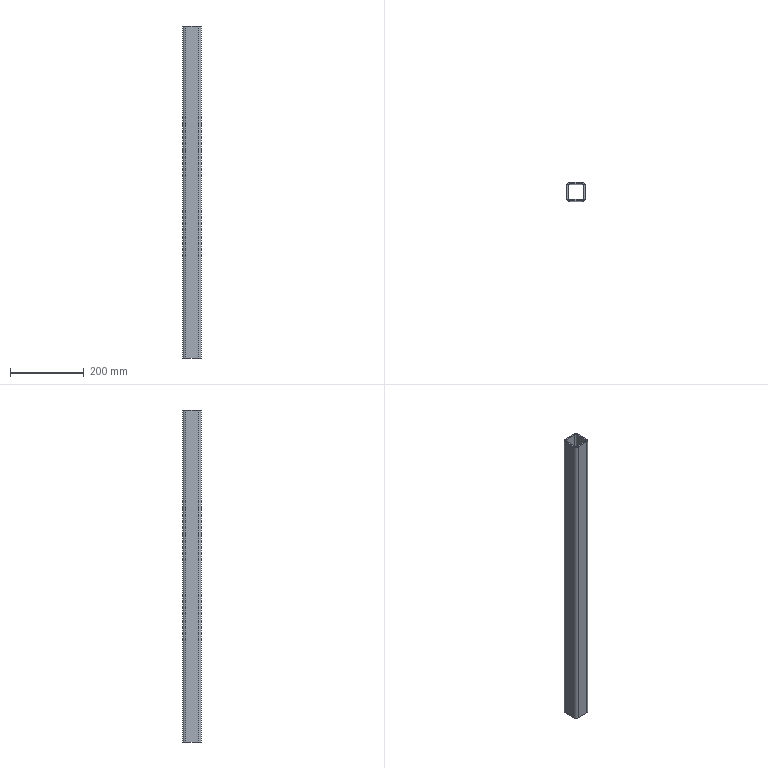Part | SolidWorks | features Extrusion 1 | 1 solid | 18 faces | box 50 x 50 x 900 mm | volume 625317 mm3 | plane 10 | cylinder 8 | commonest cylinder face diameters 8 x4 16 x4
STEP:
#1=CARTESIAN_POINT('',(17.,-25.,450.));
#2=VERTEX_POINT('',#1);
#3=CARTESIAN_POINT('',(25.,-17.,450.));
#4=VERTEX_POINT('',#3);
#5=CARTESIAN_POINT('',(17.,-17.,450.));
#6=DIRECTION('',(0.,0.,1.));
#7=DIRECTION('',(1.,0.,0.));
#8=AXIS2_PLACEMENT_3D('',#5,#6,#7);
#9=CIRCLE('',#8,8.);
#10=EDGE_CURVE('',#2,#4,#9,.T.);
#11=ORIENTED_EDGE('',*,*,#10,.T.);
#12=CARTESIAN_POINT('',(25.,17.,450.));
#13=VERTEX_POINT('',#12);
#14=CARTESIAN_POINT('',(25.,-17.,450.));
#15=DIRECTION('',(0.,1.,0.));
#16=VECTOR('',#15,1000.);
#17=LINE('',#14,#16);
#18=EDGE_CURVE('',#4,#13,#17,.T.);
#19=ORIENTED_EDGE('',*,*,#18,.T.);
#20=CARTESIAN_POINT('',(17.,25.,450.));
#21=VERTEX_POINT('',#20);
#22=CARTESIAN_POINT('',(17.,17.,450.));
#23=DIRECTION('',(0.,0.,1.));
#24=DIRECTION('',(-1.,0.,0.));
#25=AXIS2_PLACEMENT_3D('',#22,#23,#24);
#26=CIRCLE('',#25,8.);
#27=EDGE_CURVE('',#13,#21,#26,.T.);
#28=ORIENTED_EDGE('',*,*,#27,.T.);
#29=CARTESIAN_POINT('',(-17.,25.,450.));
#30=VERTEX_POINT('',#29);
#31=CARTESIAN_POINT('',(-17.,25.,450.));
#32=DIRECTION('',(-1.,0.,0.));
#33=VECTOR('',#32,1000.);
#34=LINE('',#31,#33);
#35=EDGE_CURVE('',#21,#30,#34,.T.);
#36=ORIENTED_EDGE('',*,*,#35,.T.);
#37=CARTESIAN_POINT('',(-25.,17.,450.));
#38=VERTEX_POINT('',#37);
#39=CARTESIAN_POINT('',(-17.,17.,450.));
#40=DIRECTION('',(0.,0.,1.));
#41=DIRECTION('',(-1.,0.,0.));
#42=AXIS2_PLACEMENT_3D('',#39,#40,#41);
#43=CIRCLE('',#42,8.);
#44=EDGE_CURVE('',#30,#38,#43,.T.);
#45=ORIENTED_EDGE('',*,*,#44,.T.);
#46=CARTESIAN_POINT('',(-25.,-17.,450.));
#47=VERTEX_POINT('',#46);
#48=CARTESIAN_POINT('',(-25.,-17.,450.));
#49=DIRECTION('',(0.,-1.,0.));
#50=VECTOR('',#49,1000.);
#51=LINE('',#48,#50);
#52=EDGE_CURVE('',#38,#47,#51,.T.);
#53=ORIENTED_EDGE('',*,*,#52,.T.);
#54=CARTESIAN_POINT('',(-17.,-25.,450.));
#55=VERTEX_POINT('',#54);
#56=CARTESIAN_POINT('',(-17.,-17.,450.));
#57=DIRECTION('',(0.,0.,1.));
#58=DIRECTION('',(-1.,0.,0.));
#59=AXIS2_PLACEMENT_3D('',#56,#57,#58);
#60=CIRCLE('',#59,8.);
#61=EDGE_CURVE('',#47,#55,#60,.T.);
#62=ORIENTED_EDGE('',*,*,#61,.T.);
#63=CARTESIAN_POINT('',(-17.,-25.,450.));
#64=DIRECTION('',(1.,0.,0.));
#65=VECTOR('',#64,1000.);
#66=LINE('',#63,#65);
#67=EDGE_CURVE('',#55,#2,#66,.T.);
#68=ORIENTED_EDGE('',*,*,#67,.T.);
#69=EDGE_LOOP('',(#11,#19,#28,#36,#45,#53,#62,#68));
#70=FACE_OUTER_BOUND('',#69,.T.);
#71=CARTESIAN_POINT('',(-21.,17.,450.));
#72=VERTEX_POINT('',#71);
#73=CARTESIAN_POINT('',(-21.,-17.,450.));
#74=VERTEX_POINT('',#73);
#75=CARTESIAN_POINT('',(-21.,-17.,450.));
#76=DIRECTION('',(0.,-1.,0.));
#77=VECTOR('',#76,1000.);
#78=LINE('',#75,#77);
#79=EDGE_CURVE('',#72,#74,#78,.T.);
#80=ORIENTED_EDGE('',*,*,#79,.F.);
#81=CARTESIAN_POINT('',(-17.,21.,450.));
#82=VERTEX_POINT('',#81);
#83=CARTESIAN_POINT('',(-17.,17.,450.));
#84=DIRECTION('',(0.,0.,1.));
#85=DIRECTION('',(-1.,0.,0.));
#86=AXIS2_PLACEMENT_3D('',#83,#84,#85);
#87=CIRCLE('',#86,4.);
#88=EDGE_CURVE('',#82,#72,#87,.T.);
#89=ORIENTED_EDGE('',*,*,#88,.F.);
#90=CARTESIAN_POINT('',(17.,21.,450.));
#91=VERTEX_POINT('',#90);
#92=CARTESIAN_POINT('',(-17.,21.,450.));
#93=DIRECTION('',(-1.,0.,0.));
#94=VECTOR('',#93,1000.);
#95=LINE('',#92,#94);
#96=EDGE_CURVE('',#91,#82,#95,.T.);
#97=ORIENTED_EDGE('',*,*,#96,.F.);
#98=CARTESIAN_POINT('',(21.,17.,450.));
#99=VERTEX_POINT('',#98);
#100=CARTESIAN_POINT('',(17.,17.,450.));
#101=DIRECTION('',(0.,0.,1.));
#102=DIRECTION('',(-1.,0.,0.));
#103=AXIS2_PLACEMENT_3D('',#100,#101,#102);
#104=CIRCLE('',#103,4.);
#105=EDGE_CURVE('',#99,#91,#104,.T.);
#106=ORIENTED_EDGE('',*,*,#105,.F.);
#107=CARTESIAN_POINT('',(21.,-17.,450.));
#108=VERTEX_POINT('',#107);
#109=CARTESIAN_POINT('',(21.,-17.,450.));
#110=DIRECTION('',(0.,1.,0.));
#111=VECTOR('',#110,1000.);
#112=LINE('',#109,#111);
#113=EDGE_CURVE('',#108,#99,#112,.T.);
#114=ORIENTED_EDGE('',*,*,#113,.F.);
#115=CARTESIAN_POINT('',(17.,-21.,450.));
#116=VERTEX_POINT('',#115);
#117=CARTESIAN_POINT('',(17.,-17.,450.));
#118=DIRECTION('',(0.,0.,1.));
#119=DIRECTION('',(1.,0.,0.));
#120=AXIS2_PLACEMENT_3D('',#117,#118,#119);
#121=CIRCLE('',#120,4.);
#122=EDGE_CURVE('',#116,#108,#121,.T.);
#123=ORIENTED_EDGE('',*,*,#122,.F.);
#124=CARTESIAN_POINT('',(-17.,-21.,450.));
#125=VERTEX_POINT('',#124);
#126=CARTESIAN_POINT('',(-17.,-21.,450.));
#127=DIRECTION('',(1.,0.,0.));
#128=VECTOR('',#127,1000.);
#129=LINE('',#126,#128);
#130=EDGE_CURVE('',#125,#116,#129,.T.);
#131=ORIENTED_EDGE('',*,*,#130,.F.);
#132=CARTESIAN_POINT('',(-17.,-17.,450.));
#133=DIRECTION('',(0.,0.,1.));
#134=DIRECTION('',(-1.,0.,0.));
#135=AXIS2_PLACEMENT_3D('',#132,#133,#134);
#136=CIRCLE('',#135,4.);
#137=EDGE_CURVE('',#74,#125,#136,.T.);
#138=ORIENTED_EDGE('',*,*,#137,.F.);
#139=EDGE_LOOP('',(#80,#89,#97,#106,#114,#123,#131,#138));
#140=FACE_BOUND('',#139,.T.);
#141=CARTESIAN_POINT('',(17.,-17.,450.));
#142=DIRECTION('',(0.,0.,1.));
#143=DIRECTION('',(1.,0.,0.));
#144=AXIS2_PLACEMENT_3D('',#141,#142,#143);
#145=PLANE('',#144);
#146=ADVANCED_FACE('',(#70,#140),#145,.T.);
#147=CARTESIAN_POINT('',(17.,-25.,-450.));
#148=VERTEX_POINT('',#147);
#149=CARTESIAN_POINT('',(25.,-17.,-450.));
#150=VERTEX_POINT('',#149);
#151=CARTESIAN_POINT('',(17.,-17.,-450.));
#152=DIRECTION('',(0.,0.,1.));
#153=DIRECTION('',(1.,0.,0.));
#154=AXIS2_PLACEMENT_3D('',#151,#152,#153);
#155=CIRCLE('',#154,8.);
#156=EDGE_CURVE('',#148,#150,#155,.T.);
#157=ORIENTED_EDGE('',*,*,#156,.F.);
#158=CARTESIAN_POINT('',(-17.,-25.,-450.));
#159=VERTEX_POINT('',#158);
#160=CARTESIAN_POINT('',(-17.,-25.,-450.));
#161=DIRECTION('',(1.,0.,0.));
#162=VECTOR('',#161,1000.);
#163=LINE('',#160,#162);
#164=EDGE_CURVE('',#159,#148,#163,.T.);
#165=ORIENTED_EDGE('',*,*,#164,.F.);
#166=CARTESIAN_POINT('',(-25.,-17.,-450.));
#167=VERTEX_POINT('',#166);
#168=CARTESIAN_POINT('',(-17.,-17.,-450.));
#169=DIRECTION('',(0.,0.,1.));
#170=DIRECTION('',(-1.,0.,0.));
#171=AXIS2_PLACEMENT_3D('',#168,#169,#170);
#172=CIRCLE('',#171,8.);
#173=EDGE_CURVE('',#167,#159,#172,.T.);
#174=ORIENTED_EDGE('',*,*,#173,.F.);
#175=CARTESIAN_POINT('',(-25.,17.,-450.));
#176=VERTEX_POINT('',#175);
#177=CARTESIAN_POINT('',(-25.,-17.,-450.));
#178=DIRECTION('',(0.,-1.,0.));
#179=VECTOR('',#178,1000.);
#180=LINE('',#177,#179);
#181=EDGE_CURVE('',#176,#167,#180,.T.);
#182=ORIENTED_EDGE('',*,*,#181,.F.);
#183=CARTESIAN_POINT('',(-17.,25.,-450.));
#184=VERTEX_POINT('',#183);
#185=CARTESIAN_POINT('',(-17.,17.,-450.));
#186=DIRECTION('',(0.,0.,1.));
#187=DIRECTION('',(-1.,0.,0.));
#188=AXIS2_PLACEMENT_3D('',#185,#186,#187);
#189=CIRCLE('',#188,8.);
#190=EDGE_CURVE('',#184,#176,#189,.T.);
#191=ORIENTED_EDGE('',*,*,#190,.F.);
#192=CARTESIAN_POINT('',(17.,25.,-450.));
#193=VERTEX_POINT('',#192);
#194=CARTESIAN_POINT('',(-17.,25.,-450.));
#195=DIRECTION('',(-1.,0.,0.));
#196=VECTOR('',#195,1000.);
#197=LINE('',#194,#196);
#198=EDGE_CURVE('',#193,#184,#197,.T.);
#199=ORIENTED_EDGE('',*,*,#198,.F.);
#200=CARTESIAN_POINT('',(25.,17.,-450.));
#201=VERTEX_POINT('',#200);
#202=CARTESIAN_POINT('',(17.,17.,-450.));
#203=DIRECTION('',(0.,0.,1.));
#204=DIRECTION('',(-1.,0.,0.));
#205=AXIS2_PLACEMENT_3D('',#202,#203,#204);
#206=CIRCLE('',#205,8.);
#207=EDGE_CURVE('',#201,#193,#206,.T.);
#208=ORIENTED_EDGE('',*,*,#207,.F.);
#209=CARTESIAN_POINT('',(25.,-17.,-450.));
#210=DIRECTION('',(0.,1.,0.));
#211=VECTOR('',#210,1000.);
#212=LINE('',#209,#211);
#213=EDGE_CURVE('',#150,#201,#212,.T.);
#214=ORIENTED_EDGE('',*,*,#213,.F.);
#215=EDGE_LOOP('',(#157,#165,#174,#182,#191,#199,#208,#214));
#216=FACE_OUTER_BOUND('',#215,.T.);
#217=CARTESIAN_POINT('',(-17.,21.,-450.));
#218=VERTEX_POINT('',#217);
#219=CARTESIAN_POINT('',(-21.,17.,-450.));
#220=VERTEX_POINT('',#219);
#221=CARTESIAN_POINT('',(-17.,17.,-450.));
#222=DIRECTION('',(0.,0.,1.));
#223=DIRECTION('',(-1.,0.,0.));
#224=AXIS2_PLACEMENT_3D('',#221,#222,#223);
#225=CIRCLE('',#224,4.);
#226=EDGE_CURVE('',#218,#220,#225,.T.);
#227=ORIENTED_EDGE('',*,*,#226,.T.);
#228=CARTESIAN_POINT('',(-21.,-17.,-450.));
#229=VERTEX_POINT('',#228);
#230=CARTESIAN_POINT('',(-21.,-17.,-450.));
#231=DIRECTION('',(0.,-1.,0.));
#232=VECTOR('',#231,1000.);
#233=LINE('',#230,#232);
#234=EDGE_CURVE('',#220,#229,#233,.T.);
#235=ORIENTED_EDGE('',*,*,#234,.T.);
#236=CARTESIAN_POINT('',(-17.,-21.,-450.));
#237=VERTEX_POINT('',#236);
#238=CARTESIAN_POINT('',(-17.,-17.,-450.));
#239=DIRECTION('',(0.,0.,1.));
#240=DIRECTION('',(-1.,0.,0.));
#241=AXIS2_PLACEMENT_3D('',#238,#239,#240);
#242=CIRCLE('',#241,4.);
#243=EDGE_CURVE('',#229,#237,#242,.T.);
#244=ORIENTED_EDGE('',*,*,#243,.T.);
#245=CARTESIAN_POINT('',(17.,-21.,-450.));
#246=VERTEX_POINT('',#245);
#247=CARTESIAN_POINT('',(-17.,-21.,-450.));
#248=DIRECTION('',(1.,0.,0.));
#249=VECTOR('',#248,1000.);
#250=LINE('',#247,#249);
#251=EDGE_CURVE('',#237,#246,#250,.T.);
#252=ORIENTED_EDGE('',*,*,#251,.T.);
#253=CARTESIAN_POINT('',(21.,-17.,-450.));
#254=VERTEX_POINT('',#253);
#255=CARTESIAN_POINT('',(17.,-17.,-450.));
#256=DIRECTION('',(0.,0.,1.));
#257=DIRECTION('',(1.,0.,0.));
#258=AXIS2_PLACEMENT_3D('',#255,#256,#257);
#259=CIRCLE('',#258,4.);
#260=EDGE_CURVE('',#246,#254,#259,.T.);
#261=ORIENTED_EDGE('',*,*,#260,.T.);
#262=CARTESIAN_POINT('',(21.,17.,-450.));
#263=VERTEX_POINT('',#262);
#264=CARTESIAN_POINT('',(21.,-17.,-450.));
#265=DIRECTION('',(0.,1.,0.));
#266=VECTOR('',#265,1000.);
#267=LINE('',#264,#266);
#268=EDGE_CURVE('',#254,#263,#267,.T.);
#269=ORIENTED_EDGE('',*,*,#268,.T.);
#270=CARTESIAN_POINT('',(17.,21.,-450.));
#271=VERTEX_POINT('',#270);
#272=CARTESIAN_POINT('',(17.,17.,-450.));
#273=DIRECTION('',(0.,0.,1.));
#274=DIRECTION('',(-1.,0.,0.));
#275=AXIS2_PLACEMENT_3D('',#272,#273,#274);
#276=CIRCLE('',#275,4.);
#277=EDGE_CURVE('',#263,#271,#276,.T.);
#278=ORIENTED_EDGE('',*,*,#277,.T.);
#279=CARTESIAN_POINT('',(-17.,21.,-450.));
#280=DIRECTION('',(-1.,0.,0.));
#281=VECTOR('',#280,1000.);
#282=LINE('',#279,#281);
#283=EDGE_CURVE('',#271,#218,#282,.T.);
#284=ORIENTED_EDGE('',*,*,#283,.T.);
#285=EDGE_LOOP('',(#227,#235,#244,#252,#261,#269,#278,#284));
#286=FACE_BOUND('',#285,.T.);
#287=CARTESIAN_POINT('',(17.,-17.,-450.));
#288=DIRECTION('',(0.,0.,1.));
#289=DIRECTION('',(1.,0.,0.));
#290=AXIS2_PLACEMENT_3D('',#287,#288,#289);
#291=PLANE('',#290);
#292=ADVANCED_FACE('',(#216,#286),#291,.F.);
#293=ORIENTED_EDGE('',*,*,#156,.T.);
#294=CARTESIAN_POINT('',(25.,-17.,450.));
#295=DIRECTION('',(0.,0.,-1.));
#296=VECTOR('',#295,1000.);
#297=LINE('',#294,#296);
#298=EDGE_CURVE('',#4,#150,#297,.T.);
#299=ORIENTED_EDGE('',*,*,#298,.F.);
#300=ORIENTED_EDGE('',*,*,#10,.F.);
#301=CARTESIAN_POINT('',(17.,-25.,450.));
#302=DIRECTION('',(0.,0.,-1.));
#303=VECTOR('',#302,1000.);
#304=LINE('',#301,#303);
#305=EDGE_CURVE('',#2,#148,#304,.T.);
#306=ORIENTED_EDGE('',*,*,#305,.T.);
#307=EDGE_LOOP('',(#293,#299,#300,#306));
#308=FACE_OUTER_BOUND('',#307,.T.);
#309=CARTESIAN_POINT('',(17.,-17.,450.));
#310=DIRECTION('',(0.,0.,-1.));
#311=DIRECTION('',(-1.,0.,0.));
#312=AXIS2_PLACEMENT_3D('',#309,#310,#311);
#313=CYLINDRICAL_SURFACE('',#312,8.);
#314=ADVANCED_FACE('',(#308),#313,.T.);
#315=ORIENTED_EDGE('',*,*,#213,.T.);
#316=CARTESIAN_POINT('',(25.,17.,450.));
#317=DIRECTION('',(0.,0.,-1.));
#318=VECTOR('',#317,1000.);
#319=LINE('',#316,#318);
#320=EDGE_CURVE('',#13,#201,#319,.T.);
#321=ORIENTED_EDGE('',*,*,#320,.F.);
#322=ORIENTED_EDGE('',*,*,#18,.F.);
#323=ORIENTED_EDGE('',*,*,#298,.T.);
#324=EDGE_LOOP('',(#315,#321,#322,#323));
#325=FACE_OUTER_BOUND('',#324,.T.);
#326=CARTESIAN_POINT('',(25.,-17.,450.));
#327=DIRECTION('',(-1.,0.,0.));
#328=DIRECTION('',(0.,0.,1.));
#329=AXIS2_PLACEMENT_3D('',#326,#327,#328);
#330=PLANE('',#329);
#331=ADVANCED_FACE('',(#325),#330,.F.);
#332=ORIENTED_EDGE('',*,*,#207,.T.);
#333=CARTESIAN_POINT('',(17.,25.,450.));
#334=DIRECTION('',(0.,0.,-1.));
#335=VECTOR('',#334,1000.);
#336=LINE('',#333,#335);
#337=EDGE_CURVE('',#21,#193,#336,.T.);
#338=ORIENTED_EDGE('',*,*,#337,.F.);
#339=ORIENTED_EDGE('',*,*,#27,.F.);
#340=ORIENTED_EDGE('',*,*,#320,.T.);
#341=EDGE_LOOP('',(#332,#338,#339,#340));
#342=FACE_OUTER_BOUND('',#341,.T.);
#343=CARTESIAN_POINT('',(17.,17.,450.));
#344=DIRECTION('',(0.,0.,-1.));
#345=DIRECTION('',(-1.,0.,0.));
#346=AXIS2_PLACEMENT_3D('',#343,#344,#345);
#347=CYLINDRICAL_SURFACE('',#346,8.);
#348=ADVANCED_FACE('',(#342),#347,.T.);
#349=ORIENTED_EDGE('',*,*,#198,.T.);
#350=CARTESIAN_POINT('',(-17.,25.,450.));
#351=DIRECTION('',(0.,0.,-1.));
#352=VECTOR('',#351,1000.);
#353=LINE('',#350,#352);
#354=EDGE_CURVE('',#30,#184,#353,.T.);
#355=ORIENTED_EDGE('',*,*,#354,.F.);
#356=ORIENTED_EDGE('',*,*,#35,.F.);
#357=ORIENTED_EDGE('',*,*,#337,.T.);
#358=EDGE_LOOP('',(#349,#355,#356,#357));
#359=FACE_OUTER_BOUND('',#358,.T.);
#360=CARTESIAN_POINT('',(-17.,25.,450.));
#361=DIRECTION('',(0.,-1.,0.));
#362=DIRECTION('',(0.,0.,-1.));
#363=AXIS2_PLACEMENT_3D('',#360,#361,#362);
#364=PLANE('',#363);
#365=ADVANCED_FACE('',(#359),#364,.F.);
#366=ORIENTED_EDGE('',*,*,#190,.T.);
#367=CARTESIAN_POINT('',(-25.,17.,450.));
#368=DIRECTION('',(0.,0.,-1.));
#369=VECTOR('',#368,1000.);
#370=LINE('',#367,#369);
#371=EDGE_CURVE('',#38,#176,#370,.T.);
#372=ORIENTED_EDGE('',*,*,#371,.F.);
#373=ORIENTED_EDGE('',*,*,#44,.F.);
#374=ORIENTED_EDGE('',*,*,#354,.T.);
#375=EDGE_LOOP('',(#366,#372,#373,#374));
#376=FACE_OUTER_BOUND('',#375,.T.);
#377=CARTESIAN_POINT('',(-17.,17.,450.));
#378=DIRECTION('',(0.,0.,-1.));
#379=DIRECTION('',(-1.,0.,0.));
#380=AXIS2_PLACEMENT_3D('',#377,#378,#379);
#381=CYLINDRICAL_SURFACE('',#380,8.);
#382=ADVANCED_FACE('',(#376),#381,.T.);
#383=ORIENTED_EDGE('',*,*,#181,.T.);
#384=CARTESIAN_POINT('',(-25.,-17.,450.));
#385=DIRECTION('',(0.,0.,-1.));
#386=VECTOR('',#385,1000.);
#387=LINE('',#384,#386);
#388=EDGE_CURVE('',#47,#167,#387,.T.);
#389=ORIENTED_EDGE('',*,*,#388,.F.);
#390=ORIENTED_EDGE('',*,*,#52,.F.);
#391=ORIENTED_EDGE('',*,*,#371,.T.);
#392=EDGE_LOOP('',(#383,#389,#390,#391));
#393=FACE_OUTER_BOUND('',#392,.T.);
#394=CARTESIAN_POINT('',(-25.,-17.,450.));
#395=DIRECTION('',(1.,0.,0.));
#396=DIRECTION('',(0.,0.,-1.));
#397=AXIS2_PLACEMENT_3D('',#394,#395,#396);
#398=PLANE('',#397);
#399=ADVANCED_FACE('',(#393),#398,.F.);
#400=ORIENTED_EDGE('',*,*,#173,.T.);
#401=CARTESIAN_POINT('',(-17.,-25.,450.));
#402=DIRECTION('',(0.,0.,-1.));
#403=VECTOR('',#402,1000.);
#404=LINE('',#401,#403);
#405=EDGE_CURVE('',#55,#159,#404,.T.);
#406=ORIENTED_EDGE('',*,*,#405,.F.);
#407=ORIENTED_EDGE('',*,*,#61,.F.);
#408=ORIENTED_EDGE('',*,*,#388,.T.);
#409=EDGE_LOOP('',(#400,#406,#407,#408));
#410=FACE_OUTER_BOUND('',#409,.T.);
#411=CARTESIAN_POINT('',(-17.,-17.,450.));
#412=DIRECTION('',(0.,0.,-1.));
#413=DIRECTION('',(-1.,0.,0.));
#414=AXIS2_PLACEMENT_3D('',#411,#412,#413);
#415=CYLINDRICAL_SURFACE('',#414,8.);
#416=ADVANCED_FACE('',(#410),#415,.T.);
#417=ORIENTED_EDGE('',*,*,#164,.T.);
#418=ORIENTED_EDGE('',*,*,#305,.F.);
#419=ORIENTED_EDGE('',*,*,#67,.F.);
#420=ORIENTED_EDGE('',*,*,#405,.T.);
#421=EDGE_LOOP('',(#417,#418,#419,#420));
#422=FACE_OUTER_BOUND('',#421,.T.);
#423=CARTESIAN_POINT('',(-17.,-25.,450.));
#424=DIRECTION('',(0.,1.,0.));
#425=DIRECTION('',(0.,0.,1.));
#426=AXIS2_PLACEMENT_3D('',#423,#424,#425);
#427=PLANE('',#426);
#428=ADVANCED_FACE('',(#422),#427,.F.);
#429=ORIENTED_EDGE('',*,*,#226,.F.);
#430=CARTESIAN_POINT('',(-17.,21.,450.));
#431=DIRECTION('',(0.,0.,-1.));
#432=VECTOR('',#431,1000.);
#433=LINE('',#430,#432);
#434=EDGE_CURVE('',#82,#218,#433,.T.);
#435=ORIENTED_EDGE('',*,*,#434,.F.);
#436=ORIENTED_EDGE('',*,*,#88,.T.);
#437=CARTESIAN_POINT('',(-21.,17.,450.));
#438=DIRECTION('',(0.,0.,-1.));
#439=VECTOR('',#438,1000.);
#440=LINE('',#437,#439);
#441=EDGE_CURVE('',#72,#220,#440,.T.);
#442=ORIENTED_EDGE('',*,*,#441,.T.);
#443=EDGE_LOOP('',(#429,#435,#436,#442));
#444=FACE_OUTER_BOUND('',#443,.T.);
#445=CARTESIAN_POINT('',(-17.,17.,450.));
#446=DIRECTION('',(0.,0.,-1.));
#447=DIRECTION('',(-1.,0.,0.));
#448=AXIS2_PLACEMENT_3D('',#445,#446,#447);
#449=CYLINDRICAL_SURFACE('',#448,4.);
#450=ADVANCED_FACE('',(#444),#449,.F.);
#451=ORIENTED_EDGE('',*,*,#234,.F.);
#452=ORIENTED_EDGE('',*,*,#441,.F.);
#453=ORIENTED_EDGE('',*,*,#79,.T.);
#454=CARTESIAN_POINT('',(-21.,-17.,450.));
#455=DIRECTION('',(0.,0.,-1.));
#456=VECTOR('',#455,1000.);
#457=LINE('',#454,#456);
#458=EDGE_CURVE('',#74,#229,#457,.T.);
#459=ORIENTED_EDGE('',*,*,#458,.T.);
#460=EDGE_LOOP('',(#451,#452,#453,#459));
#461=FACE_OUTER_BOUND('',#460,.T.);
#462=CARTESIAN_POINT('',(-21.,-17.,450.));
#463=DIRECTION('',(1.,0.,0.));
#464=DIRECTION('',(0.,0.,-1.));
#465=AXIS2_PLACEMENT_3D('',#462,#463,#464);
#466=PLANE('',#465);
#467=ADVANCED_FACE('',(#461),#466,.T.);
#468=ORIENTED_EDGE('',*,*,#243,.F.);
#469=ORIENTED_EDGE('',*,*,#458,.F.);
#470=ORIENTED_EDGE('',*,*,#137,.T.);
#471=CARTESIAN_POINT('',(-17.,-21.,450.));
#472=DIRECTION('',(0.,0.,-1.));
#473=VECTOR('',#472,1000.);
#474=LINE('',#471,#473);
#475=EDGE_CURVE('',#125,#237,#474,.T.);
#476=ORIENTED_EDGE('',*,*,#475,.T.);
#477=EDGE_LOOP('',(#468,#469,#470,#476));
#478=FACE_OUTER_BOUND('',#477,.T.);
#479=CARTESIAN_POINT('',(-17.,-17.,450.));
#480=DIRECTION('',(0.,0.,-1.));
#481=DIRECTION('',(-1.,0.,0.));
#482=AXIS2_PLACEMENT_3D('',#479,#480,#481);
#483=CYLINDRICAL_SURFACE('',#482,4.);
#484=ADVANCED_FACE('',(#478),#483,.F.);
#485=ORIENTED_EDGE('',*,*,#251,.F.);
#486=ORIENTED_EDGE('',*,*,#475,.F.);
#487=ORIENTED_EDGE('',*,*,#130,.T.);
#488=CARTESIAN_POINT('',(17.,-21.,450.));
#489=DIRECTION('',(0.,0.,-1.));
#490=VECTOR('',#489,1000.);
#491=LINE('',#488,#490);
#492=EDGE_CURVE('',#116,#246,#491,.T.);
#493=ORIENTED_EDGE('',*,*,#492,.T.);
#494=EDGE_LOOP('',(#485,#486,#487,#493));
#495=FACE_OUTER_BOUND('',#494,.T.);
#496=CARTESIAN_POINT('',(-17.,-21.,450.));
#497=DIRECTION('',(0.,1.,0.));
#498=DIRECTION('',(0.,0.,1.));
#499=AXIS2_PLACEMENT_3D('',#496,#497,#498);
#500=PLANE('',#499);
#501=ADVANCED_FACE('',(#495),#500,.T.);
#502=ORIENTED_EDGE('',*,*,#260,.F.);
#503=ORIENTED_EDGE('',*,*,#492,.F.);
#504=ORIENTED_EDGE('',*,*,#122,.T.);
#505=CARTESIAN_POINT('',(21.,-17.,450.));
#506=DIRECTION('',(0.,0.,-1.));
#507=VECTOR('',#506,1000.);
#508=LINE('',#505,#507);
#509=EDGE_CURVE('',#108,#254,#508,.T.);
#510=ORIENTED_EDGE('',*,*,#509,.T.);
#511=EDGE_LOOP('',(#502,#503,#504,#510));
#512=FACE_OUTER_BOUND('',#511,.T.);
#513=CARTESIAN_POINT('',(17.,-17.,450.));
#514=DIRECTION('',(0.,0.,-1.));
#515=DIRECTION('',(-1.,0.,0.));
#516=AXIS2_PLACEMENT_3D('',#513,#514,#515);
#517=CYLINDRICAL_SURFACE('',#516,4.);
#518=ADVANCED_FACE('',(#512),#517,.F.);
#519=ORIENTED_EDGE('',*,*,#268,.F.);
#520=ORIENTED_EDGE('',*,*,#509,.F.);
#521=ORIENTED_EDGE('',*,*,#113,.T.);
#522=CARTESIAN_POINT('',(21.,17.,450.));
#523=DIRECTION('',(0.,0.,-1.));
#524=VECTOR('',#523,1000.);
#525=LINE('',#522,#524);
#526=EDGE_CURVE('',#99,#263,#525,.T.);
#527=ORIENTED_EDGE('',*,*,#526,.T.);
#528=EDGE_LOOP('',(#519,#520,#521,#527));
#529=FACE_OUTER_BOUND('',#528,.T.);
#530=CARTESIAN_POINT('',(21.,-17.,450.));
#531=DIRECTION('',(-1.,0.,0.));
#532=DIRECTION('',(0.,0.,1.));
#533=AXIS2_PLACEMENT_3D('',#530,#531,#532);
#534=PLANE('',#533);
#535=ADVANCED_FACE('',(#529),#534,.T.);
#536=ORIENTED_EDGE('',*,*,#277,.F.);
#537=ORIENTED_EDGE('',*,*,#526,.F.);
#538=ORIENTED_EDGE('',*,*,#105,.T.);
#539=CARTESIAN_POINT('',(17.,21.,450.));
#540=DIRECTION('',(0.,0.,-1.));
#541=VECTOR('',#540,1000.);
#542=LINE('',#539,#541);
#543=EDGE_CURVE('',#91,#271,#542,.T.);
#544=ORIENTED_EDGE('',*,*,#543,.T.);
#545=EDGE_LOOP('',(#536,#537,#538,#544));
#546=FACE_OUTER_BOUND('',#545,.T.);
#547=CARTESIAN_POINT('',(17.,17.,450.));
#548=DIRECTION('',(0.,0.,-1.));
#549=DIRECTION('',(-1.,0.,0.));
#550=AXIS2_PLACEMENT_3D('',#547,#548,#549);
#551=CYLINDRICAL_SURFACE('',#550,4.);
#552=ADVANCED_FACE('',(#546),#551,.F.);
#553=ORIENTED_EDGE('',*,*,#283,.F.);
#554=ORIENTED_EDGE('',*,*,#543,.F.);
#555=ORIENTED_EDGE('',*,*,#96,.T.);
#556=ORIENTED_EDGE('',*,*,#434,.T.);
#557=EDGE_LOOP('',(#553,#554,#555,#556));
#558=FACE_OUTER_BOUND('',#557,.T.);
#559=CARTESIAN_POINT('',(-17.,21.,450.));
#560=DIRECTION('',(0.,-1.,0.));
#561=DIRECTION('',(0.,0.,-1.));
#562=AXIS2_PLACEMENT_3D('',#559,#560,#561);
#563=PLANE('',#562);
#564=ADVANCED_FACE('',(#558),#563,.T.);
#565=CLOSED_SHELL('',(#146,#292,#314,#331,#348,#365,#382,#399,#416,#428,#450,#467,#484,#501,#518,#535,#552,#564));
#566=MANIFOLD_SOLID_BREP('',#565);
#567=CARTESIAN_POINT('',(0.,0.,0.));
#568=DIRECTION('',(0.,0.,1.));
#569=DIRECTION('',(1.,0.,0.));
#570=AXIS2_PLACEMENT_3D('',#567,#568,#569);
#571=(LENGTH_UNIT()NAMED_UNIT(*)SI_UNIT(.MILLI.,.METRE.));
#572=UNCERTAINTY_MEASURE_WITH_UNIT(LENGTH_MEASURE(0.00001),#571,'','');
#573=(NAMED_UNIT(*)PLANE_ANGLE_UNIT()SI_UNIT($,.RADIAN.));
#574=(NAMED_UNIT(*)SI_UNIT($,.STERADIAN.)SOLID_ANGLE_UNIT());
#575=(GEOMETRIC_REPRESENTATION_CONTEXT(3)GLOBAL_UNCERTAINTY_ASSIGNED_CONTEXT((#572))GLOBAL_UNIT_ASSIGNED_CONTEXT((#571,#573,#574))REPRESENTATION_CONTEXT('',''));
#576=ADVANCED_BREP_SHAPE_REPRESENTATION('',(#566,#570),#575);